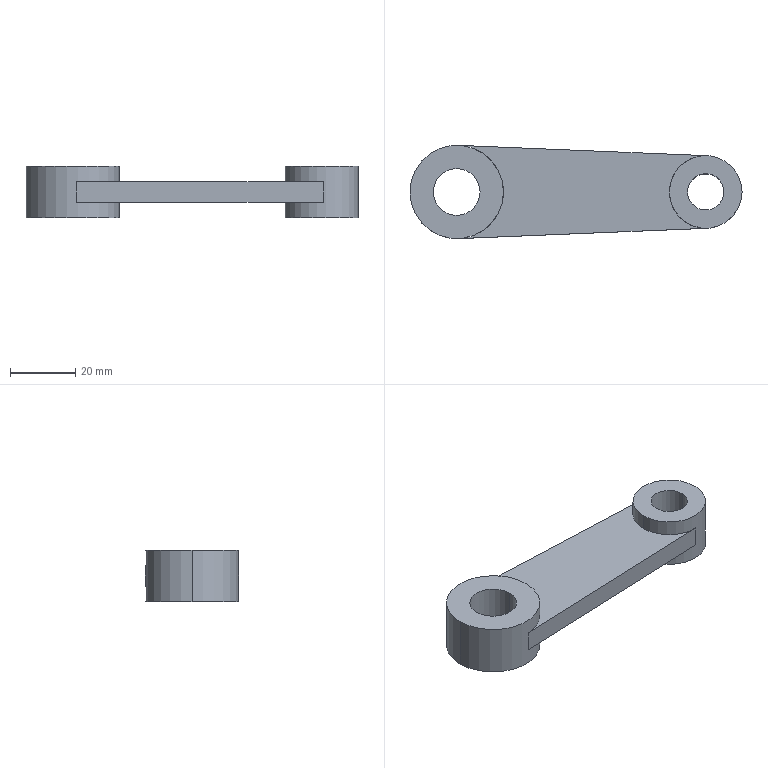Part | SolidWorks | features ICE 2, Extrusion 1 | 3 solids | 19 faces | box 101.6 x 28.575 x 15.875 mm | volume 21274 mm3 | cylinder 11 | plane 8 | commonest cylinder face diameters 22.225 x4 28.575 x3 11.125 x2 14.3 x2
STEP:
#1=CARTESIAN_POINT('',(-0.2815,0.,0.625));
#2=VERTEX_POINT('',#1);
#3=CARTESIAN_POINT('',(0.2815,0.,0.625));
#4=VERTEX_POINT('',#3);
#5=CARTESIAN_POINT('',(0.,0.,0.625));
#6=DIRECTION('',(0.,0.,1.));
#7=DIRECTION('',(1.,0.,0.));
#8=AXIS2_PLACEMENT_3D('',#5,#6,#7);
#9=CIRCLE('',#8,0.2815);
#10=EDGE_CURVE('',#2,#4,#9,.T.);
#11=ORIENTED_EDGE('',*,*,#10,.T.);
#12=CARTESIAN_POINT('',(0.2815,0.,0.));
#13=VERTEX_POINT('',#12);
#14=CARTESIAN_POINT('',(0.2815,0.,0.625));
#15=DIRECTION('',(0.,0.,-1.));
#16=VECTOR('',#15,39.37);
#17=LINE('',#14,#16);
#18=EDGE_CURVE('',#4,#13,#17,.T.);
#19=ORIENTED_EDGE('',*,*,#18,.T.);
#20=CARTESIAN_POINT('',(-0.2815,0.,0.));
#21=VERTEX_POINT('',#20);
#22=CARTESIAN_POINT('',(0.,0.,0.));
#23=DIRECTION('',(0.,0.,1.));
#24=DIRECTION('',(1.,0.,0.));
#25=AXIS2_PLACEMENT_3D('',#22,#23,#24);
#26=CIRCLE('',#25,0.2815);
#27=EDGE_CURVE('',#21,#13,#26,.T.);
#28=ORIENTED_EDGE('',*,*,#27,.F.);
#29=CARTESIAN_POINT('',(-0.2815,0.,0.625));
#30=DIRECTION('',(0.,0.,-1.));
#31=VECTOR('',#30,39.37);
#32=LINE('',#29,#31);
#33=EDGE_CURVE('',#2,#21,#32,.T.);
#34=ORIENTED_EDGE('',*,*,#33,.F.);
#35=EDGE_LOOP('',(#11,#19,#28,#34));
#36=FACE_OUTER_BOUND('',#35,.T.);
#37=CARTESIAN_POINT('',(0.,0.,0.625));
#38=DIRECTION('',(0.,0.,-1.));
#39=DIRECTION('',(-1.,0.,0.));
#40=AXIS2_PLACEMENT_3D('',#37,#38,#39);
#41=CYLINDRICAL_SURFACE('',#40,0.2815);
#42=ADVANCED_FACE('',(#36),#41,.F.);
#43=CARTESIAN_POINT('',(0.5625,0.,0.625));
#44=VERTEX_POINT('',#43);
#45=CARTESIAN_POINT('',(-0.5625,0.,0.625));
#46=VERTEX_POINT('',#45);
#47=CARTESIAN_POINT('',(0.,0.,0.625));
#48=DIRECTION('',(0.,0.,1.));
#49=DIRECTION('',(1.,0.,0.));
#50=AXIS2_PLACEMENT_3D('',#47,#48,#49);
#51=CIRCLE('',#50,0.5625);
#52=EDGE_CURVE('',#44,#46,#51,.T.);
#53=ORIENTED_EDGE('',*,*,#52,.F.);
#54=CARTESIAN_POINT('',(0.5625,0.,0.));
#55=VERTEX_POINT('',#54);
#56=CARTESIAN_POINT('',(0.5625,0.,0.625));
#57=DIRECTION('',(0.,0.,-1.));
#58=VECTOR('',#57,39.37);
#59=LINE('',#56,#58);
#60=EDGE_CURVE('',#44,#55,#59,.T.);
#61=ORIENTED_EDGE('',*,*,#60,.T.);
#62=CARTESIAN_POINT('',(-0.5625,0.,0.));
#63=VERTEX_POINT('',#62);
#64=CARTESIAN_POINT('',(0.,0.,0.));
#65=DIRECTION('',(0.,0.,1.));
#66=DIRECTION('',(1.,0.,0.));
#67=AXIS2_PLACEMENT_3D('',#64,#65,#66);
#68=CIRCLE('',#67,0.5625);
#69=EDGE_CURVE('',#55,#63,#68,.T.);
#70=ORIENTED_EDGE('',*,*,#69,.T.);
#71=CARTESIAN_POINT('',(-0.5625,0.,0.625));
#72=DIRECTION('',(0.,0.,-1.));
#73=VECTOR('',#72,39.37);
#74=LINE('',#71,#73);
#75=EDGE_CURVE('',#46,#63,#74,.T.);
#76=ORIENTED_EDGE('',*,*,#75,.F.);
#77=EDGE_LOOP('',(#53,#61,#70,#76));
#78=FACE_OUTER_BOUND('',#77,.T.);
#79=CARTESIAN_POINT('',(0.,0.,0.625));
#80=DIRECTION('',(0.,0.,-1.));
#81=DIRECTION('',(-1.,0.,0.));
#82=AXIS2_PLACEMENT_3D('',#79,#80,#81);
#83=CYLINDRICAL_SURFACE('',#82,0.5625);
#84=ADVANCED_FACE('',(#78),#83,.T.);
#85=CARTESIAN_POINT('',(0.,0.,0.625));
#86=DIRECTION('',(0.,0.,1.));
#87=DIRECTION('',(1.,0.,0.));
#88=AXIS2_PLACEMENT_3D('',#85,#86,#87);
#89=CIRCLE('',#88,0.5625);
#90=EDGE_CURVE('',#46,#44,#89,.T.);
#91=ORIENTED_EDGE('',*,*,#90,.T.);
#92=ORIENTED_EDGE('',*,*,#52,.T.);
#93=EDGE_LOOP('',(#91,#92));
#94=FACE_OUTER_BOUND('',#93,.T.);
#95=ORIENTED_EDGE('',*,*,#10,.F.);
#96=CARTESIAN_POINT('',(0.,0.,0.625));
#97=DIRECTION('',(0.,0.,1.));
#98=DIRECTION('',(1.,0.,0.));
#99=AXIS2_PLACEMENT_3D('',#96,#97,#98);
#100=CIRCLE('',#99,0.2815);
#101=EDGE_CURVE('',#4,#2,#100,.T.);
#102=ORIENTED_EDGE('',*,*,#101,.F.);
#103=EDGE_LOOP('',(#95,#102));
#104=FACE_BOUND('',#103,.T.);
#105=CARTESIAN_POINT('',(0.,0.,0.625));
#106=DIRECTION('',(0.,0.,1.));
#107=DIRECTION('',(1.,0.,0.));
#108=AXIS2_PLACEMENT_3D('',#105,#106,#107);
#109=PLANE('',#108);
#110=ADVANCED_FACE('',(#94,#104),#109,.T.);
#111=CARTESIAN_POINT('',(0.,0.,0.));
#112=DIRECTION('',(0.,0.,1.));
#113=DIRECTION('',(1.,0.,0.));
#114=AXIS2_PLACEMENT_3D('',#111,#112,#113);
#115=CIRCLE('',#114,0.5625);
#116=EDGE_CURVE('',#63,#55,#115,.T.);
#117=ORIENTED_EDGE('',*,*,#116,.F.);
#118=ORIENTED_EDGE('',*,*,#69,.F.);
#119=EDGE_LOOP('',(#117,#118));
#120=FACE_OUTER_BOUND('',#119,.T.);
#121=ORIENTED_EDGE('',*,*,#27,.T.);
#122=CARTESIAN_POINT('',(0.,0.,0.));
#123=DIRECTION('',(0.,0.,1.));
#124=DIRECTION('',(1.,0.,0.));
#125=AXIS2_PLACEMENT_3D('',#122,#123,#124);
#126=CIRCLE('',#125,0.2815);
#127=EDGE_CURVE('',#13,#21,#126,.T.);
#128=ORIENTED_EDGE('',*,*,#127,.T.);
#129=EDGE_LOOP('',(#121,#128));
#130=FACE_BOUND('',#129,.T.);
#131=CARTESIAN_POINT('',(0.,0.,0.));
#132=DIRECTION('',(0.,0.,1.));
#133=DIRECTION('',(1.,0.,0.));
#134=AXIS2_PLACEMENT_3D('',#131,#132,#133);
#135=PLANE('',#134);
#136=ADVANCED_FACE('',(#120,#130),#135,.F.);
#137=ORIENTED_EDGE('',*,*,#60,.F.);
#138=ORIENTED_EDGE('',*,*,#90,.F.);
#139=ORIENTED_EDGE('',*,*,#75,.T.);
#140=ORIENTED_EDGE('',*,*,#116,.T.);
#141=EDGE_LOOP('',(#137,#138,#139,#140));
#142=FACE_OUTER_BOUND('',#141,.T.);
#143=CARTESIAN_POINT('',(0.,0.,0.625));
#144=DIRECTION('',(0.,0.,-1.));
#145=DIRECTION('',(-1.,0.,0.));
#146=AXIS2_PLACEMENT_3D('',#143,#144,#145);
#147=CYLINDRICAL_SURFACE('',#146,0.5625);
#148=ADVANCED_FACE('',(#142),#147,.T.);
#149=ORIENTED_EDGE('',*,*,#18,.F.);
#150=ORIENTED_EDGE('',*,*,#101,.T.);
#151=ORIENTED_EDGE('',*,*,#33,.T.);
#152=ORIENTED_EDGE('',*,*,#127,.F.);
#153=EDGE_LOOP('',(#149,#150,#151,#152));
#154=FACE_OUTER_BOUND('',#153,.T.);
#155=CARTESIAN_POINT('',(0.,0.,0.625));
#156=DIRECTION('',(0.,0.,-1.));
#157=DIRECTION('',(-1.,0.,0.));
#158=AXIS2_PLACEMENT_3D('',#155,#156,#157);
#159=CYLINDRICAL_SURFACE('',#158,0.2815);
#160=ADVANCED_FACE('',(#154),#159,.F.);
#161=CLOSED_SHELL('',(#42,#84,#110,#136,#148,#160));
#162=MANIFOLD_SOLID_BREP('',#161);
#163=CARTESIAN_POINT('',(2.781,0.,0.));
#164=VERTEX_POINT('',#163);
#165=CARTESIAN_POINT('',(3.219,0.,0.));
#166=VERTEX_POINT('',#165);
#167=CARTESIAN_POINT('',(3.,0.,0.));
#168=DIRECTION('',(0.,0.,1.));
#169=DIRECTION('',(1.,0.,0.));
#170=AXIS2_PLACEMENT_3D('',#167,#168,#169);
#171=CIRCLE('',#170,0.219);
#172=EDGE_CURVE('',#164,#166,#171,.T.);
#173=ORIENTED_EDGE('',*,*,#172,.F.);
#174=CARTESIAN_POINT('',(2.781,0.,0.625));
#175=VERTEX_POINT('',#174);
#176=CARTESIAN_POINT('',(2.781,0.,0.));
#177=DIRECTION('',(0.,0.,1.));
#178=VECTOR('',#177,39.37);
#179=LINE('',#176,#178);
#180=EDGE_CURVE('',#164,#175,#179,.T.);
#181=ORIENTED_EDGE('',*,*,#180,.T.);
#182=CARTESIAN_POINT('',(3.219,0.,0.625));
#183=VERTEX_POINT('',#182);
#184=CARTESIAN_POINT('',(3.,0.,0.625));
#185=DIRECTION('',(0.,0.,1.));
#186=DIRECTION('',(1.,0.,0.));
#187=AXIS2_PLACEMENT_3D('',#184,#185,#186);
#188=CIRCLE('',#187,0.219);
#189=EDGE_CURVE('',#175,#183,#188,.T.);
#190=ORIENTED_EDGE('',*,*,#189,.T.);
#191=CARTESIAN_POINT('',(3.219,0.,0.));
#192=DIRECTION('',(0.,0.,1.));
#193=VECTOR('',#192,39.37);
#194=LINE('',#191,#193);
#195=EDGE_CURVE('',#166,#183,#194,.T.);
#196=ORIENTED_EDGE('',*,*,#195,.F.);
#197=EDGE_LOOP('',(#173,#181,#190,#196));
#198=FACE_OUTER_BOUND('',#197,.T.);
#199=CARTESIAN_POINT('',(3.,0.,0.));
#200=DIRECTION('',(0.,0.,1.));
#201=DIRECTION('',(1.,0.,0.));
#202=AXIS2_PLACEMENT_3D('',#199,#200,#201);
#203=CYLINDRICAL_SURFACE('',#202,0.219);
#204=ADVANCED_FACE('',(#198),#203,.F.);
#205=CARTESIAN_POINT('',(3.438,0.,0.));
#206=VERTEX_POINT('',#205);
#207=CARTESIAN_POINT('',(2.563,0.,0.));
#208=VERTEX_POINT('',#207);
#209=CARTESIAN_POINT('',(3.,0.,0.));
#210=DIRECTION('',(0.,0.,1.));
#211=DIRECTION('',(1.,0.,0.));
#212=AXIS2_PLACEMENT_3D('',#209,#210,#211);
#213=CIRCLE('',#212,0.4375);
#214=EDGE_CURVE('',#206,#208,#213,.T.);
#215=ORIENTED_EDGE('',*,*,#214,.T.);
#216=CARTESIAN_POINT('',(2.563,0.,0.625));
#217=VERTEX_POINT('',#216);
#218=CARTESIAN_POINT('',(2.563,0.,0.));
#219=DIRECTION('',(0.,0.,1.));
#220=VECTOR('',#219,39.37);
#221=LINE('',#218,#220);
#222=EDGE_CURVE('',#208,#217,#221,.T.);
#223=ORIENTED_EDGE('',*,*,#222,.T.);
#224=CARTESIAN_POINT('',(3.438,0.,0.625));
#225=VERTEX_POINT('',#224);
#226=CARTESIAN_POINT('',(3.,0.,0.625));
#227=DIRECTION('',(0.,0.,1.));
#228=DIRECTION('',(1.,0.,0.));
#229=AXIS2_PLACEMENT_3D('',#226,#227,#228);
#230=CIRCLE('',#229,0.4375);
#231=EDGE_CURVE('',#225,#217,#230,.T.);
#232=ORIENTED_EDGE('',*,*,#231,.F.);
#233=CARTESIAN_POINT('',(3.438,0.,0.));
#234=DIRECTION('',(0.,0.,1.));
#235=VECTOR('',#234,39.37);
#236=LINE('',#233,#235);
#237=EDGE_CURVE('',#206,#225,#236,.T.);
#238=ORIENTED_EDGE('',*,*,#237,.F.);
#239=EDGE_LOOP('',(#215,#223,#232,#238));
#240=FACE_OUTER_BOUND('',#239,.T.);
#241=CARTESIAN_POINT('',(3.,0.,0.));
#242=DIRECTION('',(0.,0.,1.));
#243=DIRECTION('',(1.,0.,0.));
#244=AXIS2_PLACEMENT_3D('',#241,#242,#243);
#245=CYLINDRICAL_SURFACE('',#244,0.4375);
#246=ADVANCED_FACE('',(#240),#245,.T.);
#247=ORIENTED_EDGE('',*,*,#222,.F.);
#248=CARTESIAN_POINT('',(3.,0.,0.));
#249=DIRECTION('',(0.,0.,1.));
#250=DIRECTION('',(1.,0.,0.));
#251=AXIS2_PLACEMENT_3D('',#248,#249,#250);
#252=CIRCLE('',#251,0.4375);
#253=EDGE_CURVE('',#208,#206,#252,.T.);
#254=ORIENTED_EDGE('',*,*,#253,.T.);
#255=ORIENTED_EDGE('',*,*,#237,.T.);
#256=CARTESIAN_POINT('',(3.,0.,0.625));
#257=DIRECTION('',(0.,0.,1.));
#258=DIRECTION('',(1.,0.,0.));
#259=AXIS2_PLACEMENT_3D('',#256,#257,#258);
#260=CIRCLE('',#259,0.4375);
#261=EDGE_CURVE('',#217,#225,#260,.T.);
#262=ORIENTED_EDGE('',*,*,#261,.F.);
#263=EDGE_LOOP('',(#247,#254,#255,#262));
#264=FACE_OUTER_BOUND('',#263,.T.);
#265=CARTESIAN_POINT('',(3.,0.,0.));
#266=DIRECTION('',(0.,0.,1.));
#267=DIRECTION('',(1.,0.,0.));
#268=AXIS2_PLACEMENT_3D('',#265,#266,#267);
#269=CYLINDRICAL_SURFACE('',#268,0.4375);
#270=ADVANCED_FACE('',(#264),#269,.T.);
#271=CARTESIAN_POINT('',(3.,0.,0.));
#272=DIRECTION('',(0.,0.,1.));
#273=DIRECTION('',(1.,0.,0.));
#274=AXIS2_PLACEMENT_3D('',#271,#272,#273);
#275=CIRCLE('',#274,0.219);
#276=EDGE_CURVE('',#166,#164,#275,.T.);
#277=ORIENTED_EDGE('',*,*,#276,.T.);
#278=ORIENTED_EDGE('',*,*,#172,.T.);
#279=EDGE_LOOP('',(#277,#278));
#280=FACE_BOUND('',#279,.T.);
#281=ORIENTED_EDGE('',*,*,#214,.F.);
#282=ORIENTED_EDGE('',*,*,#253,.F.);
#283=EDGE_LOOP('',(#281,#282));
#284=FACE_OUTER_BOUND('',#283,.T.);
#285=CARTESIAN_POINT('',(3.,0.,0.));
#286=DIRECTION('',(0.,0.,1.));
#287=DIRECTION('',(1.,0.,0.));
#288=AXIS2_PLACEMENT_3D('',#285,#286,#287);
#289=PLANE('',#288);
#290=ADVANCED_FACE('',(#280,#284),#289,.F.);
#291=CARTESIAN_POINT('',(3.,0.,0.625));
#292=DIRECTION('',(0.,0.,1.));
#293=DIRECTION('',(1.,0.,0.));
#294=AXIS2_PLACEMENT_3D('',#291,#292,#293);
#295=CIRCLE('',#294,0.219);
#296=EDGE_CURVE('',#183,#175,#295,.T.);
#297=ORIENTED_EDGE('',*,*,#296,.F.);
#298=ORIENTED_EDGE('',*,*,#189,.F.);
#299=EDGE_LOOP('',(#297,#298));
#300=FACE_BOUND('',#299,.T.);
#301=ORIENTED_EDGE('',*,*,#231,.T.);
#302=ORIENTED_EDGE('',*,*,#261,.T.);
#303=EDGE_LOOP('',(#301,#302));
#304=FACE_OUTER_BOUND('',#303,.T.);
#305=CARTESIAN_POINT('',(3.,0.,0.625));
#306=DIRECTION('',(0.,0.,1.));
#307=DIRECTION('',(1.,0.,0.));
#308=AXIS2_PLACEMENT_3D('',#305,#306,#307);
#309=PLANE('',#308);
#310=ADVANCED_FACE('',(#300,#304),#309,.T.);
#311=ORIENTED_EDGE('',*,*,#180,.F.);
#312=ORIENTED_EDGE('',*,*,#276,.F.);
#313=ORIENTED_EDGE('',*,*,#195,.T.);
#314=ORIENTED_EDGE('',*,*,#296,.T.);
#315=EDGE_LOOP('',(#311,#312,#313,#314));
#316=FACE_OUTER_BOUND('',#315,.T.);
#317=CARTESIAN_POINT('',(3.,0.,0.));
#318=DIRECTION('',(0.,0.,1.));
#319=DIRECTION('',(1.,0.,0.));
#320=AXIS2_PLACEMENT_3D('',#317,#318,#319);
#321=CYLINDRICAL_SURFACE('',#320,0.219);
#322=ADVANCED_FACE('',(#316),#321,.F.);
#323=CLOSED_SHELL('',(#204,#246,#270,#290,#310,#322));
#324=MANIFOLD_SOLID_BREP('',#323);
#325=CARTESIAN_POINT('',(3.018,0.4371,0.4375));
#326=VERTEX_POINT('',#325);
#327=CARTESIAN_POINT('',(2.563,0.,0.4375));
#328=VERTEX_POINT('',#327);
#329=CARTESIAN_POINT('',(3.,0.,0.4375));
#330=DIRECTION('',(0.,0.,1.));
#331=DIRECTION('',(1.,0.,0.));
#332=AXIS2_PLACEMENT_3D('',#329,#330,#331);
#333=CIRCLE('',#332,0.4375);
#334=EDGE_CURVE('',#326,#328,#333,.T.);
#335=ORIENTED_EDGE('',*,*,#334,.T.);
#336=CARTESIAN_POINT('',(2.563,0.,0.1875));
#337=VERTEX_POINT('',#336);
#338=CARTESIAN_POINT('',(2.563,0.,0.4375));
#339=DIRECTION('',(0.,0.,-1.));
#340=VECTOR('',#339,39.37);
#341=LINE('',#338,#340);
#342=EDGE_CURVE('',#328,#337,#341,.T.);
#343=ORIENTED_EDGE('',*,*,#342,.T.);
#344=CARTESIAN_POINT('',(3.018,0.4371,0.1875));
#345=VERTEX_POINT('',#344);
#346=CARTESIAN_POINT('',(3.,0.,0.1875));
#347=DIRECTION('',(0.,0.,1.));
#348=DIRECTION('',(1.,0.,0.));
#349=AXIS2_PLACEMENT_3D('',#346,#347,#348);
#350=CIRCLE('',#349,0.4375);
#351=EDGE_CURVE('',#345,#337,#350,.T.);
#352=ORIENTED_EDGE('',*,*,#351,.F.);
#353=CARTESIAN_POINT('',(3.018,0.4371,0.4375));
#354=DIRECTION('',(0.,0.,-1.));
#355=VECTOR('',#354,39.37);
#356=LINE('',#353,#355);
#357=EDGE_CURVE('',#326,#345,#356,.T.);
#358=ORIENTED_EDGE('',*,*,#357,.F.);
#359=EDGE_LOOP('',(#335,#343,#352,#358));
#360=FACE_OUTER_BOUND('',#359,.T.);
#361=CARTESIAN_POINT('',(3.,0.,0.4375));
#362=DIRECTION('',(0.,0.,-1.));
#363=DIRECTION('',(-1.,0.,0.));
#364=AXIS2_PLACEMENT_3D('',#361,#362,#363);
#365=CYLINDRICAL_SURFACE('',#364,0.4375);
#366=ADVANCED_FACE('',(#360),#365,.F.);
#367=CARTESIAN_POINT('',(0.04665,-0.5606,0.1875));
#368=VERTEX_POINT('',#367);
#369=CARTESIAN_POINT('',(0.04665,0.5606,0.1875));
#370=VERTEX_POINT('',#369);
#371=CARTESIAN_POINT('',(0.,0.,0.1875));
#372=DIRECTION('',(0.,0.,1.));
#373=DIRECTION('',(1.,0.,0.));
#374=AXIS2_PLACEMENT_3D('',#371,#372,#373);
#375=CIRCLE('',#374,0.5625);
#376=EDGE_CURVE('',#368,#370,#375,.T.);
#377=ORIENTED_EDGE('',*,*,#376,.F.);
#378=CARTESIAN_POINT('',(0.04665,-0.5606,0.4375));
#379=VERTEX_POINT('',#378);
#380=CARTESIAN_POINT('',(0.04665,-0.5606,0.4375));
#381=DIRECTION('',(0.,0.,-1.));
#382=VECTOR('',#381,39.37);
#383=LINE('',#380,#382);
#384=EDGE_CURVE('',#379,#368,#383,.T.);
#385=ORIENTED_EDGE('',*,*,#384,.F.);
#386=CARTESIAN_POINT('',(0.04665,0.5606,0.4375));
#387=VERTEX_POINT('',#386);
#388=CARTESIAN_POINT('',(0.,0.,0.4375));
#389=DIRECTION('',(0.,0.,1.));
#390=DIRECTION('',(1.,0.,0.));
#391=AXIS2_PLACEMENT_3D('',#388,#389,#390);
#392=CIRCLE('',#391,0.5625);
#393=EDGE_CURVE('',#379,#387,#392,.T.);
#394=ORIENTED_EDGE('',*,*,#393,.T.);
#395=CARTESIAN_POINT('',(0.04665,0.5606,0.4375));
#396=DIRECTION('',(0.,0.,-1.));
#397=VECTOR('',#396,39.37);
#398=LINE('',#395,#397);
#399=EDGE_CURVE('',#387,#370,#398,.T.);
#400=ORIENTED_EDGE('',*,*,#399,.T.);
#401=EDGE_LOOP('',(#377,#385,#394,#400));
#402=FACE_OUTER_BOUND('',#401,.T.);
#403=CARTESIAN_POINT('',(0.,0.,0.4375));
#404=DIRECTION('',(0.,0.,-1.));
#405=DIRECTION('',(-1.,0.,0.));
#406=AXIS2_PLACEMENT_3D('',#403,#404,#405);
#407=CYLINDRICAL_SURFACE('',#406,0.5625);
#408=ADVANCED_FACE('',(#402),#407,.F.);
#409=CARTESIAN_POINT('',(3.018,-0.4371,0.1875));
#410=VERTEX_POINT('',#409);
#411=CARTESIAN_POINT('',(0.02333,-0.5615,0.1875));
#412=DIRECTION('',(-0.9991,-0.04151,0.));
#413=VECTOR('',#412,39.37);
#414=LINE('',#411,#413);
#415=EDGE_CURVE('',#410,#368,#414,.T.);
#416=ORIENTED_EDGE('',*,*,#415,.F.);
#417=CARTESIAN_POINT('',(3.018,-0.4371,0.4375));
#418=VERTEX_POINT('',#417);
#419=CARTESIAN_POINT('',(3.018,-0.4371,0.4375));
#420=DIRECTION('',(0.,0.,-1.));
#421=VECTOR('',#420,39.37);
#422=LINE('',#419,#421);
#423=EDGE_CURVE('',#418,#410,#422,.T.);
#424=ORIENTED_EDGE('',*,*,#423,.F.);
#425=CARTESIAN_POINT('',(0.02333,-0.5615,0.4375));
#426=DIRECTION('',(-0.9991,-0.04151,0.));
#427=VECTOR('',#426,39.37);
#428=LINE('',#425,#427);
#429=EDGE_CURVE('',#418,#379,#428,.T.);
#430=ORIENTED_EDGE('',*,*,#429,.T.);
#431=ORIENTED_EDGE('',*,*,#384,.T.);
#432=EDGE_LOOP('',(#416,#424,#430,#431));
#433=FACE_OUTER_BOUND('',#432,.T.);
#434=CARTESIAN_POINT('',(0.02333,-0.5615,0.4375));
#435=DIRECTION('',(0.04151,-0.9991,0.));
#436=DIRECTION('',(0.9991,0.04151,0.));
#437=AXIS2_PLACEMENT_3D('',#434,#435,#436);
#438=PLANE('',#437);
#439=ADVANCED_FACE('',(#433),#438,.T.);
#440=ORIENTED_EDGE('',*,*,#342,.F.);
#441=CARTESIAN_POINT('',(3.,0.,0.4375));
#442=DIRECTION('',(0.,0.,1.));
#443=DIRECTION('',(1.,0.,0.));
#444=AXIS2_PLACEMENT_3D('',#441,#442,#443);
#445=CIRCLE('',#444,0.4375);
#446=EDGE_CURVE('',#328,#418,#445,.T.);
#447=ORIENTED_EDGE('',*,*,#446,.T.);
#448=ORIENTED_EDGE('',*,*,#423,.T.);
#449=CARTESIAN_POINT('',(3.,0.,0.1875));
#450=DIRECTION('',(0.,0.,1.));
#451=DIRECTION('',(1.,0.,0.));
#452=AXIS2_PLACEMENT_3D('',#449,#450,#451);
#453=CIRCLE('',#452,0.4375);
#454=EDGE_CURVE('',#337,#410,#453,.T.);
#455=ORIENTED_EDGE('',*,*,#454,.F.);
#456=EDGE_LOOP('',(#440,#447,#448,#455));
#457=FACE_OUTER_BOUND('',#456,.T.);
#458=CARTESIAN_POINT('',(3.,0.,0.4375));
#459=DIRECTION('',(0.,0.,-1.));
#460=DIRECTION('',(-1.,0.,0.));
#461=AXIS2_PLACEMENT_3D('',#458,#459,#460);
#462=CYLINDRICAL_SURFACE('',#461,0.4375);
#463=ADVANCED_FACE('',(#457),#462,.F.);
#464=CARTESIAN_POINT('',(0.02333,0.5615,0.1875));
#465=DIRECTION('',(0.9991,-0.04151,0.));
#466=VECTOR('',#465,39.37);
#467=LINE('',#464,#466);
#468=EDGE_CURVE('',#370,#345,#467,.T.);
#469=ORIENTED_EDGE('',*,*,#468,.F.);
#470=ORIENTED_EDGE('',*,*,#399,.F.);
#471=CARTESIAN_POINT('',(0.02333,0.5615,0.4375));
#472=DIRECTION('',(0.9991,-0.04151,0.));
#473=VECTOR('',#472,39.37);
#474=LINE('',#471,#473);
#475=EDGE_CURVE('',#387,#326,#474,.T.);
#476=ORIENTED_EDGE('',*,*,#475,.T.);
#477=ORIENTED_EDGE('',*,*,#357,.T.);
#478=EDGE_LOOP('',(#469,#470,#476,#477));
#479=FACE_OUTER_BOUND('',#478,.T.);
#480=CARTESIAN_POINT('',(0.02333,0.5615,0.4375));
#481=DIRECTION('',(0.04151,0.9991,0.));
#482=DIRECTION('',(-0.9991,0.04151,0.));
#483=AXIS2_PLACEMENT_3D('',#480,#481,#482);
#484=PLANE('',#483);
#485=ADVANCED_FACE('',(#479),#484,.T.);
#486=ORIENTED_EDGE('',*,*,#393,.F.);
#487=ORIENTED_EDGE('',*,*,#429,.F.);
#488=ORIENTED_EDGE('',*,*,#446,.F.);
#489=ORIENTED_EDGE('',*,*,#334,.F.);
#490=ORIENTED_EDGE('',*,*,#475,.F.);
#491=EDGE_LOOP('',(#486,#487,#488,#489,#490));
#492=FACE_OUTER_BOUND('',#491,.T.);
#493=CARTESIAN_POINT('',(0.,0.,0.4375));
#494=DIRECTION('',(0.,0.,1.));
#495=DIRECTION('',(1.,0.,0.));
#496=AXIS2_PLACEMENT_3D('',#493,#494,#495);
#497=PLANE('',#496);
#498=ADVANCED_FACE('',(#492),#497,.T.);
#499=ORIENTED_EDGE('',*,*,#376,.T.);
#500=ORIENTED_EDGE('',*,*,#468,.T.);
#501=ORIENTED_EDGE('',*,*,#351,.T.);
#502=ORIENTED_EDGE('',*,*,#454,.T.);
#503=ORIENTED_EDGE('',*,*,#415,.T.);
#504=EDGE_LOOP('',(#499,#500,#501,#502,#503));
#505=FACE_OUTER_BOUND('',#504,.T.);
#506=CARTESIAN_POINT('',(0.,0.,0.1875));
#507=DIRECTION('',(0.,0.,1.));
#508=DIRECTION('',(1.,0.,0.));
#509=AXIS2_PLACEMENT_3D('',#506,#507,#508);
#510=PLANE('',#509);
#511=ADVANCED_FACE('',(#505),#510,.F.);
#512=CLOSED_SHELL('',(#366,#408,#439,#463,#485,#498,#511));
#513=MANIFOLD_SOLID_BREP('',#512);
#514=CARTESIAN_POINT('',(0.,0.,0.));
#515=DIRECTION('',(0.,0.,1.));
#516=DIRECTION('',(1.,0.,0.));
#517=AXIS2_PLACEMENT_3D('',#514,#515,#516);
#518=(LENGTH_UNIT()NAMED_UNIT(*)SI_UNIT($,.METRE.));
#519=LENGTH_MEASURE_WITH_UNIT(LENGTH_MEASURE(0.0254),#518);
#520=DIMENSIONAL_EXPONENTS(1.,0.,0.,0.,0.,0.,0.);
#521=(CONVERSION_BASED_UNIT('INCH',#519)LENGTH_UNIT()NAMED_UNIT(#520));
#522=UNCERTAINTY_MEASURE_WITH_UNIT(LENGTH_MEASURE(0.00001),#521,'','');
#523=(NAMED_UNIT(*)PLANE_ANGLE_UNIT()SI_UNIT($,.RADIAN.));
#524=(NAMED_UNIT(*)SI_UNIT($,.STERADIAN.)SOLID_ANGLE_UNIT());
#525=(GEOMETRIC_REPRESENTATION_CONTEXT(3)GLOBAL_UNCERTAINTY_ASSIGNED_CONTEXT((#522))GLOBAL_UNIT_ASSIGNED_CONTEXT((#521,#523,#524))REPRESENTATION_CONTEXT('',''));
#526=ADVANCED_BREP_SHAPE_REPRESENTATION('',(#162,#324,#513,#517),#525);